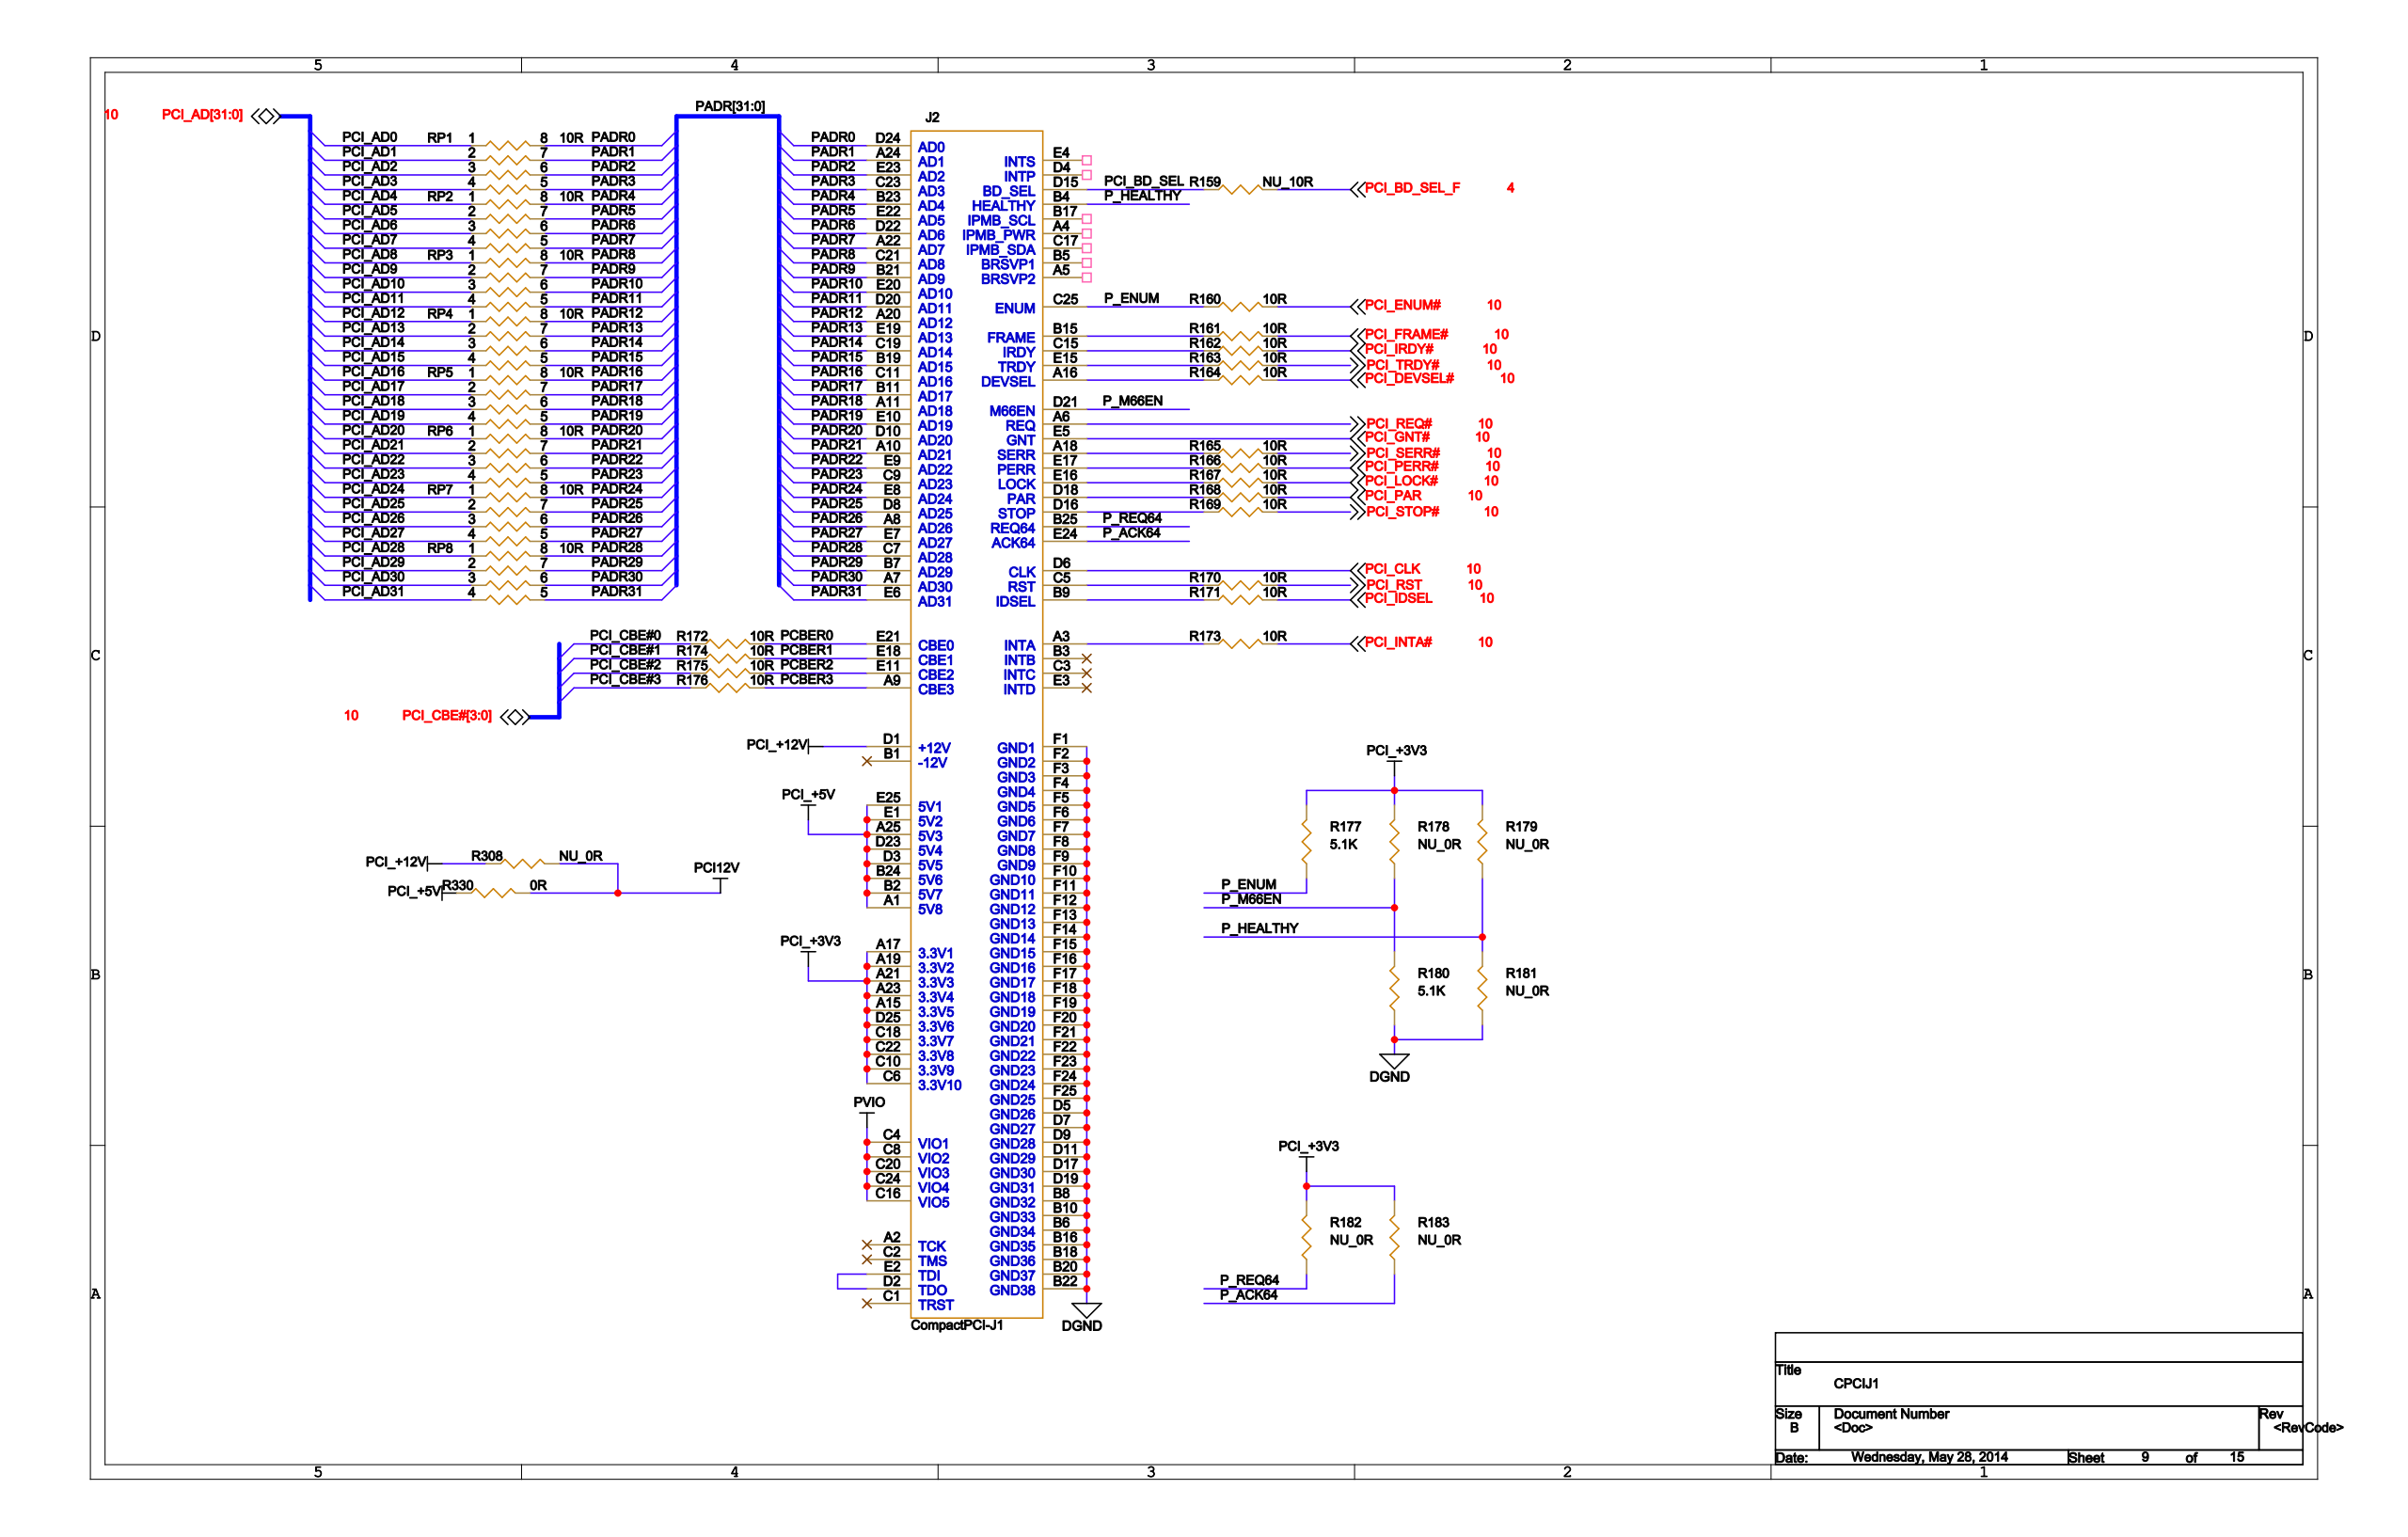Circuit board | Cadence Allegro | 669 parts | 806 nets | one sheet of the schematic
Parts on this sheet (reference | value | footprint):
J2 | CompactPCI-J1 | CPCI_J1_4
R159 | NU_10R | R0603
R160 | 10R | R0603
R161 | 10R | R0603
R162 | 10R | R0603
R163 | 10R | R0603
R164 | 10R | R0603
R165 | 10R | R0603
R166 | 10R | R0603
R167 | 10R | R0603
R168 | 10R | R0603
R169 | 10R | R0603
R170 | 10R | R0603
R171 | 10R | R0603
R172 | 10R | R0603
R173 | 10R | R0603
R174 | 10R | R0603
R175 | 10R | R0603
R176 | 10R | R0603
R177 | 5.1K | R0603
R178 | NU_0R | R0603
R179 | NU_0R | R0603
R180 | 5.1K | R0603
R181 | NU_0R | R0603
R182 | NU_0R | R0603
R183 | NU_0R | R0603
R308 | NU_0R | R1210
R330 | 0R | R1210
RP1 | 10R | 8P4R0603
RP2 | 10R | 8P4R0603
RP3 | 10R | 8P4R0603
RP4 | 10R | 8P4R0603
RP5 | 10R | 8P4R0603
RP6 | 10R | 8P4R0603
RP7 | 10R | 8P4R0603
RP8 | 10R | 8P4R0603
Nets of these parts (net: part-pin ...):
DGND: R180-1 R181-1 J2-B6 J2-B8 J2-B10 J2-B16 J2-B18 J2-B20 J2-B22 J2-D5 J2-D7 J2-D9 J2-D11 J2-D17 J2-D19 J2-F1 J2-F2 J2-F3 J2-F4 J2-F5 J2-F6 J2-F7 J2-F8 J2-F9 J2-F10 J2-F11 J2-F12 J2-F13 J2-F14 J2-F15 J2-F16 J2-F17 J2-F18 J2-F19 J2-F20 J2-F21 J2-F22 J2-F23 J2-F24 J2-F25
PCI_BD_SEL_F: R159-2
P_M66EN: R178-1 R180-2 J2-D21
PCI_+3V3: R177-2 R178-2 R179-2 R182-2 R183-2 J2-A15 J2-A17 J2-A19 J2-A21 J2-A23 J2-C6 J2-C10 J2-C18 J2-C22 J2-D25
P_HEALTHY: R179-1 R181-2 J2-B4
P_REQ64: R182-1 J2-B25
P_ACK64: R183-1 J2-E24
PCI_BD_SEL: R159-1 J2-D15
PCI_+5V: R330-1 J2-A1 J2-A25 J2-B2 J2-B24 J2-D3 J2-D23 J2-E1 J2-E25
P_ENUM: R160-1 R177-1 J2-C25
PCI_ENUM#: R160-2
N47193606: R161-1 J2-B15
PCI_FRAME#: R161-2
N47193615: R162-1 J2-C15
PCI_IRDY#: R162-2
N47193551: R163-1 J2-E15
PCI_TRDY#: R163-2
N47193560: R164-1 J2-A16
PCI_DEVSEL#: R164-2
N47193573: R165-1 J2-A18
PCI_SERR#: R165-2
N47193575: R166-1 J2-E17
PCI_PERR#: R166-2
N47193646: R167-1 J2-E16
PCI_LOCK#: R167-2
N47193571: R168-1 J2-D18
PCI_PAR: R168-2
N47193579: R169-1 J2-D16
PCI_STOP#: R169-2
N47193611: R170-1 J2-C5
PCI_RST: R170-2
N47193613: R171-1 J2-B9
PCI_IDSEL: R171-2
PCI_CBE#0: R172-1
PCBER0: R172-2 J2-E21
N47193577: R173-1 J2-A3
PCI_INTA#: R173-2
PCI_CBE#1: R174-1
PCBER1: R174-2 J2-E18
PCI_CBE#2: R175-1
PCBER2: R175-2 J2-E11
PCI_CBE#3: R176-1
PCBER3: R176-2 J2-A9
PCI_+12V: R308-1 J2-D1
PCI12V: R308-2 R330-2
PCI_AD0: RP1-1
PADR0: RP1-8 J2-D24
PCI_AD1: RP1-2
PADR1: RP1-7 J2-A24
PCI_AD2: RP1-3
PADR2: RP1-6 J2-E23
PCI_AD3: RP1-4
PADR3: RP1-5 J2-C23
PCI_AD4: RP2-1
PADR4: RP2-8 J2-B23
PCI_AD5: RP2-2
PADR5: RP2-7 J2-E22
PCI_AD6: RP2-3
PADR6: RP2-6 J2-D22
PCI_AD7: RP2-4
PADR7: RP2-5 J2-A22
PCI_AD8: RP3-1
PADR8: RP3-8 J2-C21
PCI_AD9: RP3-2
PADR9: RP3-7 J2-B21
PCI_AD10: RP3-3
PADR10: RP3-6 J2-E20
PCI_AD11: RP3-4
PADR11: RP3-5 J2-D20
PCI_AD12: RP4-1
PADR12: RP4-8 J2-A20
PCI_AD13: RP4-2
PADR13: RP4-7 J2-E19
PCI_AD14: RP4-3
PADR14: RP4-6 J2-C19
PCI_AD15: RP4-4
PADR15: RP4-5 J2-B19
PCI_AD16: RP5-1
PADR16: RP5-8 J2-C11
PCI_AD17: RP5-2
PADR17: RP5-7 J2-B11
PCI_AD18: RP5-3
PADR18: RP5-6 J2-A11
PCI_AD19: RP5-4
PADR19: RP5-5 J2-E10
PCI_AD20: RP6-1
PADR20: RP6-8 J2-D10
PCI_AD21: RP6-2
PADR21: RP6-7 J2-A10
PCI_AD22: RP6-3
PADR22: RP6-6 J2-E9
PCI_AD23: RP6-4
PADR23: RP6-5 J2-C9
PCI_AD24: RP7-1
PADR24: RP7-8 J2-E8
PCI_AD25: RP7-2
PADR25: RP7-7 J2-D8
PCI_AD26: RP7-3
PADR26: RP7-6 J2-A8
PCI_AD27: RP7-4
PADR27: RP7-5 J2-E7
PCI_AD28: RP8-1
PADR28: RP8-8 J2-C7
PCI_AD29: RP8-2
PADR29: RP8-7 J2-B7
PCI_AD30: RP8-3
PADR30: RP8-6 J2-A7
PCI_AD31: RP8-4
PADR31: RP8-5 J2-E6
PCI_CLK: J2-D6
PCI_GNT#: J2-E5
PCI_REQ#: J2-A6
PVIO: J2-C4 J2-C8 J2-C16 J2-C20 J2-C24